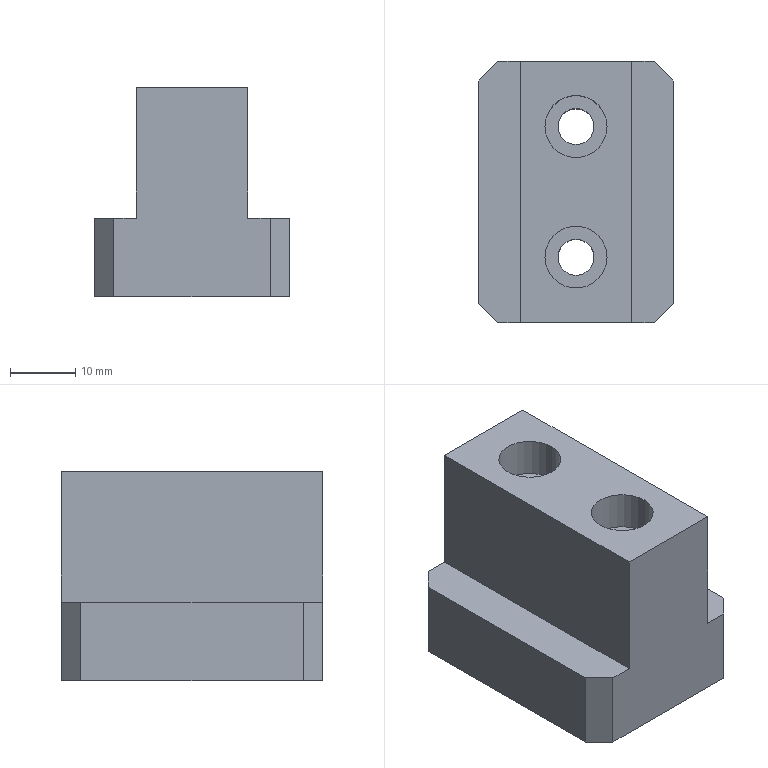Part | Creo | 1 solid | 24 faces | box 30 x 40 x 32 mm | volume 25698 mm3 | plane 16 | cylinder 8 | commonest cylinder face diameters 5.5 x4 9.5 x4
STEP:
#1=CARTESIAN_POINT('',(0.,0.,0.));
#2=DIRECTION('',(0.,0.,1.));
#3=DIRECTION('',(1.,0.,0.));
#4=AXIS2_PLACEMENT_3D('',#1,#2,#3);
#5=CARTESIAN_POINT('',(-123.5,148.,19.5));
#6=VERTEX_POINT('',#5);
#7=CARTESIAN_POINT('',(-140.5,148.,19.5));
#8=VERTEX_POINT('',#7);
#9=CARTESIAN_POINT('',(-123.5,148.,19.5));
#10=DIRECTION('',(-1.,0.,0.));
#11=VECTOR('',#10,17.);
#12=LINE('',#9,#11);
#13=EDGE_CURVE('',#6,#8,#12,.T.);
#14=ORIENTED_EDGE('',*,*,#13,.T.);
#15=CARTESIAN_POINT('',(-140.5,188.,19.5));
#16=VERTEX_POINT('',#15);
#17=CARTESIAN_POINT('',(-140.5,148.,19.5));
#18=DIRECTION('',(0.,1.,0.));
#19=VECTOR('',#18,40.);
#20=LINE('',#17,#19);
#21=EDGE_CURVE('',#8,#16,#20,.T.);
#22=ORIENTED_EDGE('',*,*,#21,.T.);
#23=CARTESIAN_POINT('',(-123.5,188.,19.5));
#24=VERTEX_POINT('',#23);
#25=CARTESIAN_POINT('',(-140.5,188.,19.5));
#26=DIRECTION('',(1.,0.,0.));
#27=VECTOR('',#26,17.);
#28=LINE('',#25,#27);
#29=EDGE_CURVE('',#16,#24,#28,.T.);
#30=ORIENTED_EDGE('',*,*,#29,.T.);
#31=CARTESIAN_POINT('',(-123.5,188.,19.5));
#32=DIRECTION('',(0.,-1.,0.));
#33=VECTOR('',#32,40.);
#34=LINE('',#31,#33);
#35=EDGE_CURVE('',#24,#6,#34,.T.);
#36=ORIENTED_EDGE('',*,*,#35,.T.);
#37=EDGE_LOOP('',(#14,#22,#30,#36));
#38=FACE_OUTER_BOUND('',#37,.F.);
#39=CARTESIAN_POINT('',(-127.25,178.,19.5));
#40=VERTEX_POINT('',#39);
#41=CARTESIAN_POINT('',(-136.75,178.,19.5));
#42=VERTEX_POINT('',#41);
#43=CARTESIAN_POINT('',(-132.,178.,19.5));
#44=DIRECTION('',(0.,0.,-1.));
#45=DIRECTION('',(1.,0.,0.));
#46=AXIS2_PLACEMENT_3D('',#43,#44,#45);
#47=CIRCLE('',#46,4.75);
#48=EDGE_CURVE('',#40,#42,#47,.T.);
#49=ORIENTED_EDGE('',*,*,#48,.F.);
#50=CARTESIAN_POINT('',(-132.,178.,19.5));
#51=DIRECTION('',(0.,0.,-1.));
#52=DIRECTION('',(-1.,0.,0.));
#53=AXIS2_PLACEMENT_3D('',#50,#51,#52);
#54=CIRCLE('',#53,4.75);
#55=EDGE_CURVE('',#42,#40,#54,.T.);
#56=ORIENTED_EDGE('',*,*,#55,.F.);
#57=EDGE_LOOP('',(#49,#56));
#58=FACE_BOUND('',#57,.F.);
#59=CARTESIAN_POINT('',(-127.25,158.,19.5));
#60=VERTEX_POINT('',#59);
#61=CARTESIAN_POINT('',(-136.75,158.,19.5));
#62=VERTEX_POINT('',#61);
#63=CARTESIAN_POINT('',(-132.,158.,19.5));
#64=DIRECTION('',(0.,0.,-1.));
#65=DIRECTION('',(1.,0.,0.));
#66=AXIS2_PLACEMENT_3D('',#63,#64,#65);
#67=CIRCLE('',#66,4.75);
#68=EDGE_CURVE('',#60,#62,#67,.T.);
#69=ORIENTED_EDGE('',*,*,#68,.F.);
#70=CARTESIAN_POINT('',(-132.,158.,19.5));
#71=DIRECTION('',(0.,0.,-1.));
#72=DIRECTION('',(-1.,0.,0.));
#73=AXIS2_PLACEMENT_3D('',#70,#71,#72);
#74=CIRCLE('',#73,4.75);
#75=EDGE_CURVE('',#62,#60,#74,.T.);
#76=ORIENTED_EDGE('',*,*,#75,.F.);
#77=EDGE_LOOP('',(#69,#76));
#78=FACE_BOUND('',#77,.F.);
#79=CARTESIAN_POINT('',(25.,303.,19.5));
#80=DIRECTION('',(0.,0.,1.));
#81=DIRECTION('',(0.,1.,0.));
#82=AXIS2_PLACEMENT_3D('',#79,#80,#81);
#83=PLANE('',#82);
#84=ADVANCED_FACE('',(#38,#58,#78),#83,.T.);
#85=CARTESIAN_POINT('',(-136.75,158.,13.5));
#86=VERTEX_POINT('',#85);
#87=CARTESIAN_POINT('',(-127.25,158.,13.5));
#88=VERTEX_POINT('',#87);
#89=CARTESIAN_POINT('',(-132.,158.,13.5));
#90=DIRECTION('',(0.,0.,1.));
#91=DIRECTION('',(-1.,0.,0.));
#92=AXIS2_PLACEMENT_3D('',#89,#90,#91);
#93=CIRCLE('',#92,4.75);
#94=EDGE_CURVE('',#86,#88,#93,.T.);
#95=ORIENTED_EDGE('',*,*,#94,.T.);
#96=CARTESIAN_POINT('',(-127.25,158.,13.5));
#97=DIRECTION('',(0.,0.,1.));
#98=VECTOR('',#97,6.);
#99=LINE('',#96,#98);
#100=EDGE_CURVE('',#88,#60,#99,.T.);
#101=ORIENTED_EDGE('',*,*,#100,.T.);
#102=ORIENTED_EDGE('',*,*,#68,.T.);
#103=CARTESIAN_POINT('',(-136.75,158.,13.5));
#104=DIRECTION('',(0.,0.,1.));
#105=VECTOR('',#104,6.);
#106=LINE('',#103,#105);
#107=EDGE_CURVE('',#86,#62,#106,.T.);
#108=ORIENTED_EDGE('',*,*,#107,.F.);
#109=EDGE_LOOP('',(#95,#101,#102,#108));
#110=FACE_OUTER_BOUND('',#109,.F.);
#111=CARTESIAN_POINT('',(-132.,158.,19.5));
#112=DIRECTION('',(0.,0.,1.));
#113=DIRECTION('',(1.,0.,0.));
#114=AXIS2_PLACEMENT_3D('',#111,#112,#113);
#115=CYLINDRICAL_SURFACE('',#114,4.75);
#116=ADVANCED_FACE('',(#110),#115,.F.);
#117=CARTESIAN_POINT('',(-132.,158.,13.5));
#118=DIRECTION('',(0.,0.,1.));
#119=DIRECTION('',(1.,0.,0.));
#120=AXIS2_PLACEMENT_3D('',#117,#118,#119);
#121=CIRCLE('',#120,4.75);
#122=EDGE_CURVE('',#88,#86,#121,.T.);
#123=ORIENTED_EDGE('',*,*,#122,.F.);
#124=ORIENTED_EDGE('',*,*,#94,.F.);
#125=EDGE_LOOP('',(#123,#124));
#126=FACE_OUTER_BOUND('',#125,.F.);
#127=CARTESIAN_POINT('',(-129.25,158.,13.5));
#128=VERTEX_POINT('',#127);
#129=CARTESIAN_POINT('',(-134.75,158.,13.5));
#130=VERTEX_POINT('',#129);
#131=CARTESIAN_POINT('',(-132.,158.,13.5));
#132=DIRECTION('',(0.,0.,-1.));
#133=DIRECTION('',(1.,0.,0.));
#134=AXIS2_PLACEMENT_3D('',#131,#132,#133);
#135=CIRCLE('',#134,2.75);
#136=EDGE_CURVE('',#128,#130,#135,.T.);
#137=ORIENTED_EDGE('',*,*,#136,.F.);
#138=CARTESIAN_POINT('',(-132.,158.,13.5));
#139=DIRECTION('',(0.,0.,-1.));
#140=DIRECTION('',(-1.,0.,0.));
#141=AXIS2_PLACEMENT_3D('',#138,#139,#140);
#142=CIRCLE('',#141,2.75);
#143=EDGE_CURVE('',#130,#128,#142,.T.);
#144=ORIENTED_EDGE('',*,*,#143,.F.);
#145=EDGE_LOOP('',(#137,#144));
#146=FACE_BOUND('',#145,.F.);
#147=CARTESIAN_POINT('',(-132.,162.75,13.5));
#148=DIRECTION('',(0.,0.,-1.));
#149=DIRECTION('',(-1.,0.,0.));
#150=AXIS2_PLACEMENT_3D('',#147,#148,#149);
#151=PLANE('',#150);
#152=ADVANCED_FACE('',(#126,#146),#151,.F.);
#153=CARTESIAN_POINT('',(-134.75,158.,-12.5));
#154=VERTEX_POINT('',#153);
#155=CARTESIAN_POINT('',(-129.25,158.,-12.5));
#156=VERTEX_POINT('',#155);
#157=CARTESIAN_POINT('',(-132.,158.,-12.5));
#158=DIRECTION('',(0.,0.,1.));
#159=DIRECTION('',(-1.,0.,0.));
#160=AXIS2_PLACEMENT_3D('',#157,#158,#159);
#161=CIRCLE('',#160,2.75);
#162=EDGE_CURVE('',#154,#156,#161,.T.);
#163=ORIENTED_EDGE('',*,*,#162,.T.);
#164=CARTESIAN_POINT('',(-129.25,158.,-12.5));
#165=DIRECTION('',(0.,0.,1.));
#166=VECTOR('',#165,26.);
#167=LINE('',#164,#166);
#168=EDGE_CURVE('',#156,#128,#167,.T.);
#169=ORIENTED_EDGE('',*,*,#168,.T.);
#170=ORIENTED_EDGE('',*,*,#136,.T.);
#171=CARTESIAN_POINT('',(-134.75,158.,-12.5));
#172=DIRECTION('',(0.,0.,1.));
#173=VECTOR('',#172,26.);
#174=LINE('',#171,#173);
#175=EDGE_CURVE('',#154,#130,#174,.T.);
#176=ORIENTED_EDGE('',*,*,#175,.F.);
#177=EDGE_LOOP('',(#163,#169,#170,#176));
#178=FACE_OUTER_BOUND('',#177,.F.);
#179=CARTESIAN_POINT('',(-132.,158.,19.5));
#180=DIRECTION('',(0.,0.,1.));
#181=DIRECTION('',(1.,0.,0.));
#182=AXIS2_PLACEMENT_3D('',#179,#180,#181);
#183=CYLINDRICAL_SURFACE('',#182,2.75);
#184=ADVANCED_FACE('',(#178),#183,.F.);
#185=CARTESIAN_POINT('',(-117.,185.,-12.5));
#186=VERTEX_POINT('',#185);
#187=CARTESIAN_POINT('',(-117.,151.,-12.5));
#188=VERTEX_POINT('',#187);
#189=CARTESIAN_POINT('',(-117.,185.,-12.5));
#190=DIRECTION('',(0.,-1.,0.));
#191=VECTOR('',#190,34.);
#192=LINE('',#189,#191);
#193=EDGE_CURVE('',#186,#188,#192,.T.);
#194=ORIENTED_EDGE('',*,*,#193,.F.);
#195=CARTESIAN_POINT('',(-120.,188.,-12.5));
#196=VERTEX_POINT('',#195);
#197=CARTESIAN_POINT('',(-120.,188.,-12.5));
#198=DIRECTION('',(0.7071,-0.7071,0.));
#199=VECTOR('',#198,4.243);
#200=LINE('',#197,#199);
#201=EDGE_CURVE('',#196,#186,#200,.T.);
#202=ORIENTED_EDGE('',*,*,#201,.F.);
#203=CARTESIAN_POINT('',(-144.,188.,-12.5));
#204=VERTEX_POINT('',#203);
#205=CARTESIAN_POINT('',(-144.,188.,-12.5));
#206=DIRECTION('',(1.,0.,0.));
#207=VECTOR('',#206,24.);
#208=LINE('',#205,#207);
#209=EDGE_CURVE('',#204,#196,#208,.T.);
#210=ORIENTED_EDGE('',*,*,#209,.F.);
#211=CARTESIAN_POINT('',(-147.,185.,-12.5));
#212=VERTEX_POINT('',#211);
#213=CARTESIAN_POINT('',(-147.,185.,-12.5));
#214=DIRECTION('',(0.7071,0.7071,0.));
#215=VECTOR('',#214,4.243);
#216=LINE('',#213,#215);
#217=EDGE_CURVE('',#212,#204,#216,.T.);
#218=ORIENTED_EDGE('',*,*,#217,.F.);
#219=CARTESIAN_POINT('',(-147.,151.,-12.5));
#220=VERTEX_POINT('',#219);
#221=CARTESIAN_POINT('',(-147.,151.,-12.5));
#222=DIRECTION('',(0.,1.,0.));
#223=VECTOR('',#222,34.);
#224=LINE('',#221,#223);
#225=EDGE_CURVE('',#220,#212,#224,.T.);
#226=ORIENTED_EDGE('',*,*,#225,.F.);
#227=CARTESIAN_POINT('',(-144.,148.,-12.5));
#228=VERTEX_POINT('',#227);
#229=CARTESIAN_POINT('',(-144.,148.,-12.5));
#230=DIRECTION('',(-0.7071,0.7071,0.));
#231=VECTOR('',#230,4.243);
#232=LINE('',#229,#231);
#233=EDGE_CURVE('',#228,#220,#232,.T.);
#234=ORIENTED_EDGE('',*,*,#233,.F.);
#235=CARTESIAN_POINT('',(-120.,148.,-12.5));
#236=VERTEX_POINT('',#235);
#237=CARTESIAN_POINT('',(-120.,148.,-12.5));
#238=DIRECTION('',(-1.,0.,0.));
#239=VECTOR('',#238,24.);
#240=LINE('',#237,#239);
#241=EDGE_CURVE('',#236,#228,#240,.T.);
#242=ORIENTED_EDGE('',*,*,#241,.F.);
#243=CARTESIAN_POINT('',(-117.,151.,-12.5));
#244=DIRECTION('',(-0.7071,-0.7071,0.));
#245=VECTOR('',#244,4.243);
#246=LINE('',#243,#245);
#247=EDGE_CURVE('',#188,#236,#246,.T.);
#248=ORIENTED_EDGE('',*,*,#247,.F.);
#249=EDGE_LOOP('',(#194,#202,#210,#218,#226,#234,#242,#248));
#250=FACE_OUTER_BOUND('',#249,.F.);
#251=CARTESIAN_POINT('',(-129.25,178.,-12.5));
#252=VERTEX_POINT('',#251);
#253=CARTESIAN_POINT('',(-134.75,178.,-12.5));
#254=VERTEX_POINT('',#253);
#255=CARTESIAN_POINT('',(-132.,178.,-12.5));
#256=DIRECTION('',(0.,0.,1.));
#257=DIRECTION('',(1.,0.,0.));
#258=AXIS2_PLACEMENT_3D('',#255,#256,#257);
#259=CIRCLE('',#258,2.75);
#260=EDGE_CURVE('',#252,#254,#259,.T.);
#261=ORIENTED_EDGE('',*,*,#260,.F.);
#262=CARTESIAN_POINT('',(-132.,178.,-12.5));
#263=DIRECTION('',(0.,0.,1.));
#264=DIRECTION('',(-1.,0.,0.));
#265=AXIS2_PLACEMENT_3D('',#262,#263,#264);
#266=CIRCLE('',#265,2.75);
#267=EDGE_CURVE('',#254,#252,#266,.T.);
#268=ORIENTED_EDGE('',*,*,#267,.F.);
#269=EDGE_LOOP('',(#261,#268));
#270=FACE_BOUND('',#269,.F.);
#271=CARTESIAN_POINT('',(-132.,158.,-12.5));
#272=DIRECTION('',(0.,0.,1.));
#273=DIRECTION('',(1.,0.,0.));
#274=AXIS2_PLACEMENT_3D('',#271,#272,#273);
#275=CIRCLE('',#274,2.75);
#276=EDGE_CURVE('',#156,#154,#275,.T.);
#277=ORIENTED_EDGE('',*,*,#276,.F.);
#278=ORIENTED_EDGE('',*,*,#162,.F.);
#279=EDGE_LOOP('',(#277,#278));
#280=FACE_BOUND('',#279,.F.);
#281=CARTESIAN_POINT('',(25.,303.,-12.5));
#282=DIRECTION('',(0.,0.,1.));
#283=DIRECTION('',(0.,1.,0.));
#284=AXIS2_PLACEMENT_3D('',#281,#282,#283);
#285=PLANE('',#284);
#286=ADVANCED_FACE('',(#250,#270,#280),#285,.F.);
#287=ORIENTED_EDGE('',*,*,#276,.T.);
#288=ORIENTED_EDGE('',*,*,#175,.T.);
#289=ORIENTED_EDGE('',*,*,#143,.T.);
#290=ORIENTED_EDGE('',*,*,#168,.F.);
#291=EDGE_LOOP('',(#287,#288,#289,#290));
#292=FACE_OUTER_BOUND('',#291,.F.);
#293=CARTESIAN_POINT('',(-132.,158.,19.5));
#294=DIRECTION('',(0.,0.,1.));
#295=DIRECTION('',(1.,0.,0.));
#296=AXIS2_PLACEMENT_3D('',#293,#294,#295);
#297=CYLINDRICAL_SURFACE('',#296,2.75);
#298=ADVANCED_FACE('',(#292),#297,.F.);
#299=ORIENTED_EDGE('',*,*,#260,.T.);
#300=CARTESIAN_POINT('',(-134.75,178.,13.5));
#301=VERTEX_POINT('',#300);
#302=CARTESIAN_POINT('',(-134.75,178.,-12.5));
#303=DIRECTION('',(0.,0.,1.));
#304=VECTOR('',#303,26.);
#305=LINE('',#302,#304);
#306=EDGE_CURVE('',#254,#301,#305,.T.);
#307=ORIENTED_EDGE('',*,*,#306,.T.);
#308=CARTESIAN_POINT('',(-129.25,178.,13.5));
#309=VERTEX_POINT('',#308);
#310=CARTESIAN_POINT('',(-132.,178.,13.5));
#311=DIRECTION('',(0.,0.,-1.));
#312=DIRECTION('',(-1.,0.,0.));
#313=AXIS2_PLACEMENT_3D('',#310,#311,#312);
#314=CIRCLE('',#313,2.75);
#315=EDGE_CURVE('',#301,#309,#314,.T.);
#316=ORIENTED_EDGE('',*,*,#315,.T.);
#317=CARTESIAN_POINT('',(-129.25,178.,-12.5));
#318=DIRECTION('',(0.,0.,1.));
#319=VECTOR('',#318,26.);
#320=LINE('',#317,#319);
#321=EDGE_CURVE('',#252,#309,#320,.T.);
#322=ORIENTED_EDGE('',*,*,#321,.F.);
#323=EDGE_LOOP('',(#299,#307,#316,#322));
#324=FACE_OUTER_BOUND('',#323,.F.);
#325=CARTESIAN_POINT('',(-132.,178.,19.5));
#326=DIRECTION('',(0.,0.,1.));
#327=DIRECTION('',(1.,0.,0.));
#328=AXIS2_PLACEMENT_3D('',#325,#326,#327);
#329=CYLINDRICAL_SURFACE('',#328,2.75);
#330=ADVANCED_FACE('',(#324),#329,.F.);
#331=ORIENTED_EDGE('',*,*,#267,.T.);
#332=ORIENTED_EDGE('',*,*,#321,.T.);
#333=CARTESIAN_POINT('',(-132.,178.,13.5));
#334=DIRECTION('',(0.,0.,-1.));
#335=DIRECTION('',(1.,0.,0.));
#336=AXIS2_PLACEMENT_3D('',#333,#334,#335);
#337=CIRCLE('',#336,2.75);
#338=EDGE_CURVE('',#309,#301,#337,.T.);
#339=ORIENTED_EDGE('',*,*,#338,.T.);
#340=ORIENTED_EDGE('',*,*,#306,.F.);
#341=EDGE_LOOP('',(#331,#332,#339,#340));
#342=FACE_OUTER_BOUND('',#341,.F.);
#343=CARTESIAN_POINT('',(-132.,178.,19.5));
#344=DIRECTION('',(0.,0.,1.));
#345=DIRECTION('',(1.,0.,0.));
#346=AXIS2_PLACEMENT_3D('',#343,#344,#345);
#347=CYLINDRICAL_SURFACE('',#346,2.75);
#348=ADVANCED_FACE('',(#342),#347,.F.);
#349=CARTESIAN_POINT('',(-127.25,178.,13.5));
#350=VERTEX_POINT('',#349);
#351=CARTESIAN_POINT('',(-136.75,178.,13.5));
#352=VERTEX_POINT('',#351);
#353=CARTESIAN_POINT('',(-132.,178.,13.5));
#354=DIRECTION('',(0.,0.,1.));
#355=DIRECTION('',(1.,0.,0.));
#356=AXIS2_PLACEMENT_3D('',#353,#354,#355);
#357=CIRCLE('',#356,4.75);
#358=EDGE_CURVE('',#350,#352,#357,.T.);
#359=ORIENTED_EDGE('',*,*,#358,.F.);
#360=CARTESIAN_POINT('',(-132.,178.,13.5));
#361=DIRECTION('',(0.,0.,1.));
#362=DIRECTION('',(-1.,0.,0.));
#363=AXIS2_PLACEMENT_3D('',#360,#361,#362);
#364=CIRCLE('',#363,4.75);
#365=EDGE_CURVE('',#352,#350,#364,.T.);
#366=ORIENTED_EDGE('',*,*,#365,.F.);
#367=EDGE_LOOP('',(#359,#366));
#368=FACE_OUTER_BOUND('',#367,.F.);
#369=ORIENTED_EDGE('',*,*,#338,.F.);
#370=ORIENTED_EDGE('',*,*,#315,.F.);
#371=EDGE_LOOP('',(#369,#370));
#372=FACE_BOUND('',#371,.F.);
#373=CARTESIAN_POINT('',(-132.,182.75,13.5));
#374=DIRECTION('',(0.,0.,-1.));
#375=DIRECTION('',(-1.,0.,0.));
#376=AXIS2_PLACEMENT_3D('',#373,#374,#375);
#377=PLANE('',#376);
#378=ADVANCED_FACE('',(#368,#372),#377,.F.);
#379=ORIENTED_EDGE('',*,*,#358,.T.);
#380=CARTESIAN_POINT('',(-136.75,178.,13.5));
#381=DIRECTION('',(0.,0.,1.));
#382=VECTOR('',#381,6.);
#383=LINE('',#380,#382);
#384=EDGE_CURVE('',#352,#42,#383,.T.);
#385=ORIENTED_EDGE('',*,*,#384,.T.);
#386=ORIENTED_EDGE('',*,*,#55,.T.);
#387=CARTESIAN_POINT('',(-127.25,178.,13.5));
#388=DIRECTION('',(0.,0.,1.));
#389=VECTOR('',#388,6.);
#390=LINE('',#387,#389);
#391=EDGE_CURVE('',#350,#40,#390,.T.);
#392=ORIENTED_EDGE('',*,*,#391,.F.);
#393=EDGE_LOOP('',(#379,#385,#386,#392));
#394=FACE_OUTER_BOUND('',#393,.F.);
#395=CARTESIAN_POINT('',(-132.,178.,19.5));
#396=DIRECTION('',(0.,0.,1.));
#397=DIRECTION('',(1.,0.,0.));
#398=AXIS2_PLACEMENT_3D('',#395,#396,#397);
#399=CYLINDRICAL_SURFACE('',#398,4.75);
#400=ADVANCED_FACE('',(#394),#399,.F.);
#401=ORIENTED_EDGE('',*,*,#365,.T.);
#402=ORIENTED_EDGE('',*,*,#391,.T.);
#403=ORIENTED_EDGE('',*,*,#48,.T.);
#404=ORIENTED_EDGE('',*,*,#384,.F.);
#405=EDGE_LOOP('',(#401,#402,#403,#404));
#406=FACE_OUTER_BOUND('',#405,.F.);
#407=CARTESIAN_POINT('',(-132.,178.,19.5));
#408=DIRECTION('',(0.,0.,1.));
#409=DIRECTION('',(1.,0.,0.));
#410=AXIS2_PLACEMENT_3D('',#407,#408,#409);
#411=CYLINDRICAL_SURFACE('',#410,4.75);
#412=ADVANCED_FACE('',(#406),#411,.F.);
#413=CARTESIAN_POINT('',(-117.,185.,-0.5));
#414=VERTEX_POINT('',#413);
#415=CARTESIAN_POINT('',(-117.,151.,-0.5));
#416=VERTEX_POINT('',#415);
#417=CARTESIAN_POINT('',(-117.,185.,-0.5));
#418=DIRECTION('',(0.,-1.,0.));
#419=VECTOR('',#418,34.);
#420=LINE('',#417,#419);
#421=EDGE_CURVE('',#414,#416,#420,.T.);
#422=ORIENTED_EDGE('',*,*,#421,.F.);
#423=CARTESIAN_POINT('',(-117.,185.,-0.5));
#424=DIRECTION('',(0.,0.,-1.));
#425=VECTOR('',#424,12.);
#426=LINE('',#423,#425);
#427=EDGE_CURVE('',#414,#186,#426,.T.);
#428=ORIENTED_EDGE('',*,*,#427,.T.);
#429=ORIENTED_EDGE('',*,*,#193,.T.);
#430=CARTESIAN_POINT('',(-117.,151.,-12.5));
#431=DIRECTION('',(0.,0.,1.));
#432=VECTOR('',#431,12.);
#433=LINE('',#430,#432);
#434=EDGE_CURVE('',#188,#416,#433,.T.);
#435=ORIENTED_EDGE('',*,*,#434,.T.);
#436=EDGE_LOOP('',(#422,#428,#429,#435));
#437=FACE_OUTER_BOUND('',#436,.F.);
#438=CARTESIAN_POINT('',(-117.,148.,-12.5));
#439=DIRECTION('',(1.,0.,0.));
#440=DIRECTION('',(0.,1.,0.));
#441=AXIS2_PLACEMENT_3D('',#438,#439,#440);
#442=PLANE('',#441);
#443=ADVANCED_FACE('',(#437),#442,.T.);
#444=CARTESIAN_POINT('',(-120.,148.,-0.5));
#445=VERTEX_POINT('',#444);
#446=CARTESIAN_POINT('',(-123.5,148.,-0.5));
#447=VERTEX_POINT('',#446);
#448=CARTESIAN_POINT('',(-120.,148.,-0.5));
#449=DIRECTION('',(-1.,0.,0.));
#450=VECTOR('',#449,3.5);
#451=LINE('',#448,#450);
#452=EDGE_CURVE('',#445,#447,#451,.T.);
#453=ORIENTED_EDGE('',*,*,#452,.T.);
#454=CARTESIAN_POINT('',(-123.5,188.,-0.5));
#455=VERTEX_POINT('',#454);
#456=CARTESIAN_POINT('',(-123.5,148.,-0.5));
#457=DIRECTION('',(0.,1.,0.));
#458=VECTOR('',#457,40.);
#459=LINE('',#456,#458);
#460=EDGE_CURVE('',#447,#455,#459,.T.);
#461=ORIENTED_EDGE('',*,*,#460,.T.);
#462=CARTESIAN_POINT('',(-120.,188.,-0.5));
#463=VERTEX_POINT('',#462);
#464=CARTESIAN_POINT('',(-120.,188.,-0.5));
#465=DIRECTION('',(-1.,0.,0.));
#466=VECTOR('',#465,3.5);
#467=LINE('',#464,#466);
#468=EDGE_CURVE('',#463,#455,#467,.T.);
#469=ORIENTED_EDGE('',*,*,#468,.F.);
#470=CARTESIAN_POINT('',(-117.,185.,-0.5));
#471=DIRECTION('',(-0.7071,0.7071,0.));
#472=VECTOR('',#471,4.243);
#473=LINE('',#470,#472);
#474=EDGE_CURVE('',#414,#463,#473,.T.);
#475=ORIENTED_EDGE('',*,*,#474,.F.);
#476=ORIENTED_EDGE('',*,*,#421,.T.);
#477=CARTESIAN_POINT('',(-120.,148.,-0.5));
#478=DIRECTION('',(0.7071,0.7071,0.));
#479=VECTOR('',#478,4.243);
#480=LINE('',#477,#479);
#481=EDGE_CURVE('',#445,#416,#480,.T.);
#482=ORIENTED_EDGE('',*,*,#481,.F.);
#483=EDGE_LOOP('',(#453,#461,#469,#475,#476,#482));
#484=FACE_OUTER_BOUND('',#483,.F.);
#485=CARTESIAN_POINT('',(-132.,168.,-0.5));
#486=DIRECTION('',(0.,0.,-1.));
#487=DIRECTION('',(0.,-1.,0.));
#488=AXIS2_PLACEMENT_3D('',#485,#486,#487);
#489=PLANE('',#488);
#490=ADVANCED_FACE('',(#484),#489,.F.);
#491=ORIENTED_EDGE('',*,*,#241,.T.);
#492=CARTESIAN_POINT('',(-144.,148.,-0.5));
#493=VERTEX_POINT('',#492);
#494=CARTESIAN_POINT('',(-144.,148.,-12.5));
#495=DIRECTION('',(0.,0.,1.));
#496=VECTOR('',#495,12.);
#497=LINE('',#494,#496);
#498=EDGE_CURVE('',#228,#493,#497,.T.);
#499=ORIENTED_EDGE('',*,*,#498,.T.);
#500=CARTESIAN_POINT('',(-140.5,148.,-0.5));
#501=VERTEX_POINT('',#500);
#502=CARTESIAN_POINT('',(-140.5,148.,-0.5));
#503=DIRECTION('',(-1.,0.,0.));
#504=VECTOR('',#503,3.5);
#505=LINE('',#502,#504);
#506=EDGE_CURVE('',#501,#493,#505,.T.);
#507=ORIENTED_EDGE('',*,*,#506,.F.);
#508=CARTESIAN_POINT('',(-140.5,148.,19.5));
#509=DIRECTION('',(0.,0.,-1.));
#510=VECTOR('',#509,20.);
#511=LINE('',#508,#510);
#512=EDGE_CURVE('',#8,#501,#511,.T.);
#513=ORIENTED_EDGE('',*,*,#512,.F.);
#514=ORIENTED_EDGE('',*,*,#13,.F.);
#515=CARTESIAN_POINT('',(-123.5,148.,19.5));
#516=DIRECTION('',(0.,0.,-1.));
#517=VECTOR('',#516,20.);
#518=LINE('',#515,#517);
#519=EDGE_CURVE('',#6,#447,#518,.T.);
#520=ORIENTED_EDGE('',*,*,#519,.T.);
#521=ORIENTED_EDGE('',*,*,#452,.F.);
#522=CARTESIAN_POINT('',(-120.,148.,-0.5));
#523=DIRECTION('',(0.,0.,-1.));
#524=VECTOR('',#523,12.);
#525=LINE('',#522,#524);
#526=EDGE_CURVE('',#445,#236,#525,.T.);
#527=ORIENTED_EDGE('',*,*,#526,.T.);
#528=EDGE_LOOP('',(#491,#499,#507,#513,#514,#520,#521,#527));
#529=FACE_OUTER_BOUND('',#528,.F.);
#530=CARTESIAN_POINT('',(-147.,148.,-12.5));
#531=DIRECTION('',(0.,-1.,0.));
#532=DIRECTION('',(0.,0.,1.));
#533=AXIS2_PLACEMENT_3D('',#530,#531,#532);
#534=PLANE('',#533);
#535=ADVANCED_FACE('',(#529),#534,.T.);
#536=ORIENTED_EDGE('',*,*,#233,.T.);
#537=CARTESIAN_POINT('',(-147.,151.,-0.5));
#538=VERTEX_POINT('',#537);
#539=CARTESIAN_POINT('',(-147.,151.,-0.5));
#540=DIRECTION('',(0.,0.,-1.));
#541=VECTOR('',#540,12.);
#542=LINE('',#539,#541);
#543=EDGE_CURVE('',#538,#220,#542,.T.);
#544=ORIENTED_EDGE('',*,*,#543,.F.);
#545=CARTESIAN_POINT('',(-147.,151.,-0.5));
#546=DIRECTION('',(0.7071,-0.7071,0.));
#547=VECTOR('',#546,4.243);
#548=LINE('',#545,#547);
#549=EDGE_CURVE('',#538,#493,#548,.T.);
#550=ORIENTED_EDGE('',*,*,#549,.T.);
#551=ORIENTED_EDGE('',*,*,#498,.F.);
#552=EDGE_LOOP('',(#536,#544,#550,#551));
#553=FACE_OUTER_BOUND('',#552,.F.);
#554=CARTESIAN_POINT('',(-147.,151.,-12.5));
#555=DIRECTION('',(0.7071,0.7071,0.));
#556=DIRECTION('',(0.,0.,1.));
#557=AXIS2_PLACEMENT_3D('',#554,#555,#556);
#558=PLANE('',#557);
#559=ADVANCED_FACE('',(#553),#558,.F.);
#560=ORIENTED_EDGE('',*,*,#225,.T.);
#561=CARTESIAN_POINT('',(-147.,185.,-0.5));
#562=VERTEX_POINT('',#561);
#563=CARTESIAN_POINT('',(-147.,185.,-12.5));
#564=DIRECTION('',(0.,0.,1.));
#565=VECTOR('',#564,12.);
#566=LINE('',#563,#565);
#567=EDGE_CURVE('',#212,#562,#566,.T.);
#568=ORIENTED_EDGE('',*,*,#567,.T.);
#569=CARTESIAN_POINT('',(-147.,151.,-0.5));
#570=DIRECTION('',(0.,1.,0.));
#571=VECTOR('',#570,34.);
#572=LINE('',#569,#571);
#573=EDGE_CURVE('',#538,#562,#572,.T.);
#574=ORIENTED_EDGE('',*,*,#573,.F.);
#575=ORIENTED_EDGE('',*,*,#543,.T.);
#576=EDGE_LOOP('',(#560,#568,#574,#575));
#577=FACE_OUTER_BOUND('',#576,.F.);
#578=CARTESIAN_POINT('',(-147.,188.,-12.5));
#579=DIRECTION('',(-1.,0.,0.));
#580=DIRECTION('',(0.,0.,1.));
#581=AXIS2_PLACEMENT_3D('',#578,#579,#580);
#582=PLANE('',#581);
#583=ADVANCED_FACE('',(#577),#582,.T.);
#584=ORIENTED_EDGE('',*,*,#217,.T.);
#585=CARTESIAN_POINT('',(-144.,188.,-0.5));
#586=VERTEX_POINT('',#585);
#587=CARTESIAN_POINT('',(-144.,188.,-0.5));
#588=DIRECTION('',(0.,0.,-1.));
#589=VECTOR('',#588,12.);
#590=LINE('',#587,#589);
#591=EDGE_CURVE('',#586,#204,#590,.T.);
#592=ORIENTED_EDGE('',*,*,#591,.F.);
#593=CARTESIAN_POINT('',(-144.,188.,-0.5));
#594=DIRECTION('',(-0.7071,-0.7071,0.));
#595=VECTOR('',#594,4.243);
#596=LINE('',#593,#595);
#597=EDGE_CURVE('',#586,#562,#596,.T.);
#598=ORIENTED_EDGE('',*,*,#597,.T.);
#599=ORIENTED_EDGE('',*,*,#567,.F.);
#600=EDGE_LOOP('',(#584,#592,#598,#599));
#601=FACE_OUTER_BOUND('',#600,.F.);
#602=CARTESIAN_POINT('',(-144.,188.,-12.5));
#603=DIRECTION('',(0.7071,-0.7071,0.));
#604=DIRECTION('',(0.,0.,1.));
#605=AXIS2_PLACEMENT_3D('',#602,#603,#604);
#606=PLANE('',#605);
#607=ADVANCED_FACE('',(#601),#606,.F.);
#608=ORIENTED_EDGE('',*,*,#468,.T.);
#609=CARTESIAN_POINT('',(-123.5,188.,19.5));
#610=DIRECTION('',(0.,0.,-1.));
#611=VECTOR('',#610,20.);
#612=LINE('',#609,#611);
#613=EDGE_CURVE('',#24,#455,#612,.T.);
#614=ORIENTED_EDGE('',*,*,#613,.F.);
#615=ORIENTED_EDGE('',*,*,#29,.F.);
#616=CARTESIAN_POINT('',(-140.5,188.,-0.5));
#617=VERTEX_POINT('',#616);
#618=CARTESIAN_POINT('',(-140.5,188.,19.5));
#619=DIRECTION('',(0.,0.,-1.));
#620=VECTOR('',#619,20.);
#621=LINE('',#618,#620);
#622=EDGE_CURVE('',#16,#617,#621,.T.);
#623=ORIENTED_EDGE('',*,*,#622,.T.);
#624=CARTESIAN_POINT('',(-140.5,188.,-0.5));
#625=DIRECTION('',(-1.,0.,0.));
#626=VECTOR('',#625,3.5);
#627=LINE('',#624,#626);
#628=EDGE_CURVE('',#617,#586,#627,.T.);
#629=ORIENTED_EDGE('',*,*,#628,.T.);
#630=ORIENTED_EDGE('',*,*,#591,.T.);
#631=ORIENTED_EDGE('',*,*,#209,.T.);
#632=CARTESIAN_POINT('',(-120.,188.,-12.5));
#633=DIRECTION('',(0.,0.,1.));
#634=VECTOR('',#633,12.);
#635=LINE('',#632,#634);
#636=EDGE_CURVE('',#196,#463,#635,.T.);
#637=ORIENTED_EDGE('',*,*,#636,.T.);
#638=EDGE_LOOP('',(#608,#614,#615,#623,#629,#630,#631,#637));
#639=FACE_OUTER_BOUND('',#638,.F.);
#640=CARTESIAN_POINT('',(-117.,188.,-12.5));
#641=DIRECTION('',(0.,1.,0.));
#642=DIRECTION('',(-1.,0.,0.));
#643=AXIS2_PLACEMENT_3D('',#640,#641,#642);
#644=PLANE('',#643);
#645=ADVANCED_FACE('',(#639),#644,.T.);
#646=ORIENTED_EDGE('',*,*,#519,.F.);
#647=ORIENTED_EDGE('',*,*,#35,.F.);
#648=ORIENTED_EDGE('',*,*,#613,.T.);
#649=ORIENTED_EDGE('',*,*,#460,.F.);
#650=EDGE_LOOP('',(#646,#647,#648,#649));
#651=FACE_OUTER_BOUND('',#650,.F.);
#652=CARTESIAN_POINT('',(-123.5,148.,-12.5));
#653=DIRECTION('',(1.,0.,0.));
#654=DIRECTION('',(0.,1.,0.));
#655=AXIS2_PLACEMENT_3D('',#652,#653,#654);
#656=PLANE('',#655);
#657=ADVANCED_FACE('',(#651),#656,.T.);
#658=ORIENTED_EDGE('',*,*,#622,.F.);
#659=ORIENTED_EDGE('',*,*,#21,.F.);
#660=ORIENTED_EDGE('',*,*,#512,.T.);
#661=CARTESIAN_POINT('',(-140.5,188.,-0.5));
#662=DIRECTION('',(0.,-1.,0.));
#663=VECTOR('',#662,40.);
#664=LINE('',#661,#663);
#665=EDGE_CURVE('',#617,#501,#664,.T.);
#666=ORIENTED_EDGE('',*,*,#665,.F.);
#667=EDGE_LOOP('',(#658,#659,#660,#666));
#668=FACE_OUTER_BOUND('',#667,.F.);
#669=CARTESIAN_POINT('',(-140.5,188.,-12.5));
#670=DIRECTION('',(-1.,0.,0.));
#671=DIRECTION('',(0.,0.,1.));
#672=AXIS2_PLACEMENT_3D('',#669,#670,#671);
#673=PLANE('',#672);
#674=ADVANCED_FACE('',(#668),#673,.T.);
#675=ORIENTED_EDGE('',*,*,#573,.T.);
#676=ORIENTED_EDGE('',*,*,#597,.F.);
#677=ORIENTED_EDGE('',*,*,#628,.F.);
#678=ORIENTED_EDGE('',*,*,#665,.T.);
#679=ORIENTED_EDGE('',*,*,#506,.T.);
#680=ORIENTED_EDGE('',*,*,#549,.F.);
#681=EDGE_LOOP('',(#675,#676,#677,#678,#679,#680));
#682=FACE_OUTER_BOUND('',#681,.F.);
#683=CARTESIAN_POINT('',(-132.,168.,-0.5));
#684=DIRECTION('',(0.,0.,-1.));
#685=DIRECTION('',(0.,-1.,0.));
#686=AXIS2_PLACEMENT_3D('',#683,#684,#685);
#687=PLANE('',#686);
#688=ADVANCED_FACE('',(#682),#687,.F.);
#689=ORIENTED_EDGE('',*,*,#201,.T.);
#690=ORIENTED_EDGE('',*,*,#427,.F.);
#691=ORIENTED_EDGE('',*,*,#474,.T.);
#692=ORIENTED_EDGE('',*,*,#636,.F.);
#693=EDGE_LOOP('',(#689,#690,#691,#692));
#694=FACE_OUTER_BOUND('',#693,.F.);
#695=CARTESIAN_POINT('',(-117.,185.,-12.5));
#696=DIRECTION('',(-0.7071,-0.7071,0.));
#697=DIRECTION('',(0.,0.,1.));
#698=AXIS2_PLACEMENT_3D('',#695,#696,#697);
#699=PLANE('',#698);
#700=ADVANCED_FACE('',(#694),#699,.F.);
#701=ORIENTED_EDGE('',*,*,#247,.T.);
#702=ORIENTED_EDGE('',*,*,#526,.F.);
#703=ORIENTED_EDGE('',*,*,#481,.T.);
#704=ORIENTED_EDGE('',*,*,#434,.F.);
#705=EDGE_LOOP('',(#701,#702,#703,#704));
#706=FACE_OUTER_BOUND('',#705,.F.);
#707=CARTESIAN_POINT('',(-120.,148.,-12.5));
#708=DIRECTION('',(-0.7071,0.7071,0.));
#709=DIRECTION('',(0.,0.,1.));
#710=AXIS2_PLACEMENT_3D('',#707,#708,#709);
#711=PLANE('',#710);
#712=ADVANCED_FACE('',(#706),#711,.F.);
#713=ORIENTED_EDGE('',*,*,#122,.T.);
#714=ORIENTED_EDGE('',*,*,#107,.T.);
#715=ORIENTED_EDGE('',*,*,#75,.T.);
#716=ORIENTED_EDGE('',*,*,#100,.F.);
#717=EDGE_LOOP('',(#713,#714,#715,#716));
#718=FACE_OUTER_BOUND('',#717,.F.);
#719=CARTESIAN_POINT('',(-132.,158.,19.5));
#720=DIRECTION('',(0.,0.,1.));
#721=DIRECTION('',(1.,0.,0.));
#722=AXIS2_PLACEMENT_3D('',#719,#720,#721);
#723=CYLINDRICAL_SURFACE('',#722,4.75);
#724=ADVANCED_FACE('',(#718),#723,.F.);
#725=CLOSED_SHELL('',(#84,#116,#152,#184,#286,#298,#330,#348,#378,#400,#412,#443,#490,#535,#559,#583,#607,#645,#657,#674,#688,#700,#712,#724));
#726=MANIFOLD_SOLID_BREP('',#725);
#727=(LENGTH_UNIT()NAMED_UNIT(*)SI_UNIT(.MILLI.,.METRE.));
#728=UNCERTAINTY_MEASURE_WITH_UNIT(LENGTH_MEASURE(0.005936),#727,'','');
#729=(NAMED_UNIT(*)PLANE_ANGLE_UNIT()SI_UNIT($,.RADIAN.));
#730=PLANE_ANGLE_MEASURE_WITH_UNIT(PLANE_ANGLE_MEASURE(0.01745),#729);
#731=(CONVERSION_BASED_UNIT('DEGREE',#730)NAMED_UNIT(*)PLANE_ANGLE_UNIT());
#732=(NAMED_UNIT(*)SI_UNIT($,.STERADIAN.)SOLID_ANGLE_UNIT());
#733=(GEOMETRIC_REPRESENTATION_CONTEXT(3)GLOBAL_UNCERTAINTY_ASSIGNED_CONTEXT((#728))GLOBAL_UNIT_ASSIGNED_CONTEXT((#727,#731,#732))REPRESENTATION_CONTEXT('',''));
#734=ADVANCED_BREP_SHAPE_REPRESENTATION('',(#4,#726),#733);